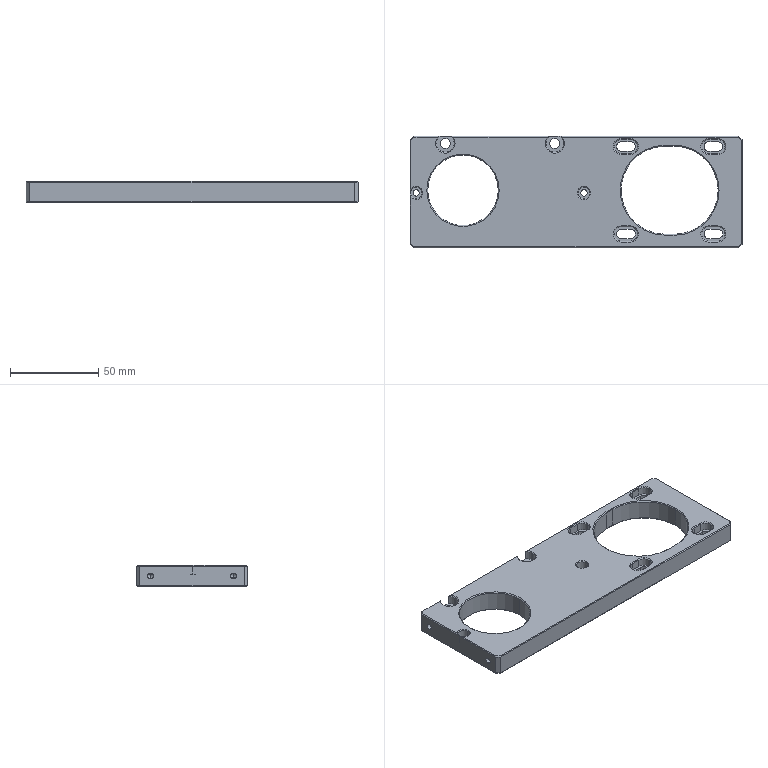Part | SolidWorks | features BaseBody 1 | 1 solid | 187 faces | box 188 x 63 x 12 mm | volume 94885 mm3 | plane 74 | cone 58 | cylinder 55 | commonest cylinder face diameters 5.5 x12 8.2 x12 3.3 x8 10 x6 3.6 x4 5.8 x4